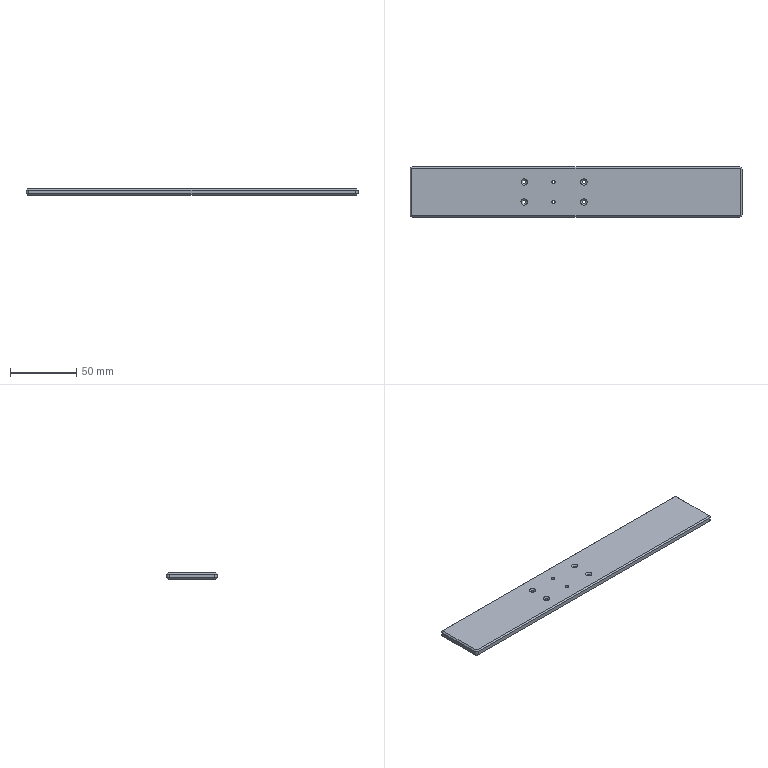NC program | NX | posted with a generic post | part box 250 x 38 x 5 mm
Lines 1 to 64 of 15324:
N10 G17 G21 G94 G90
(ZLEVEL_PROFILE , TOOL : D10)
N12 T02 M6
N14 G54
N16 G17 G0 G90 X46.558 Y-24.1 S6500 M3
N18 G43 Z35. H2
N20 Z6.5
N22 G94 G1 X0. Z4.06 F1000.
N24 X-123. F2000.
N26 G2 X-130.1 Y-17. R7.1
N28 G1 Y17.
N30 G2 X-123. Y24.1 R7.1
N32 G1 X123.
N34 G2 X130.1 Y17. R7.1
N36 G1 Y-17.
N38 G2 X123. Y-24.1 R7.1
N40 G1 X0.
N42 X-53.853 Z3.12
N44 X-123.
N46 G2 X-130.1 Y-17. R7.1
N48 G1 Y17.
N50 G2 X-123. Y24.1 R7.1
N52 G1 X123.
N54 G2 X130.1 Y17. R7.1
N56 G1 Y-17.
N58 G2 X123. Y-24.1 R7.1
N60 G1 X0.
N62 X-53.853 Z2.18
N64 X-123.
N66 G2 X-130.1 Y-17. R7.1
N68 G1 Y17.
N70 G2 X-123. Y24.1 R7.1
N72 G1 X123.
N74 G2 X130.1 Y17. R7.1
N76 G1 Y-17.
N78 G2 X123. Y-24.1 R7.1
N80 G1 X0.
N82 X-53.853 Z1.24
N84 X-123.
N86 G2 X-130.1 Y-17. R7.1
N88 G1 Y17.
N90 G2 X-123. Y24.1 R7.1
N92 G1 X123.
N94 G2 X130.1 Y17. R7.1
N96 G1 Y-17.
N98 G2 X123. Y-24.1 R7.1
N100 G1 X0.
N102 X-53.853 Z0.3
N104 X-123.
N106 G2 X-130.1 Y-17. R7.1
N108 G1 Y17.
N110 G2 X-123. Y24.1 R7.1
N112 G1 X123.
N114 G2 X130.1 Y17. R7.1
N116 G1 Y-17.
N118 G2 X123. Y-24.1 R7.1
N120 G1 X-53.853
N122 Z1.8
N124 G0 Z35.
N126 M5